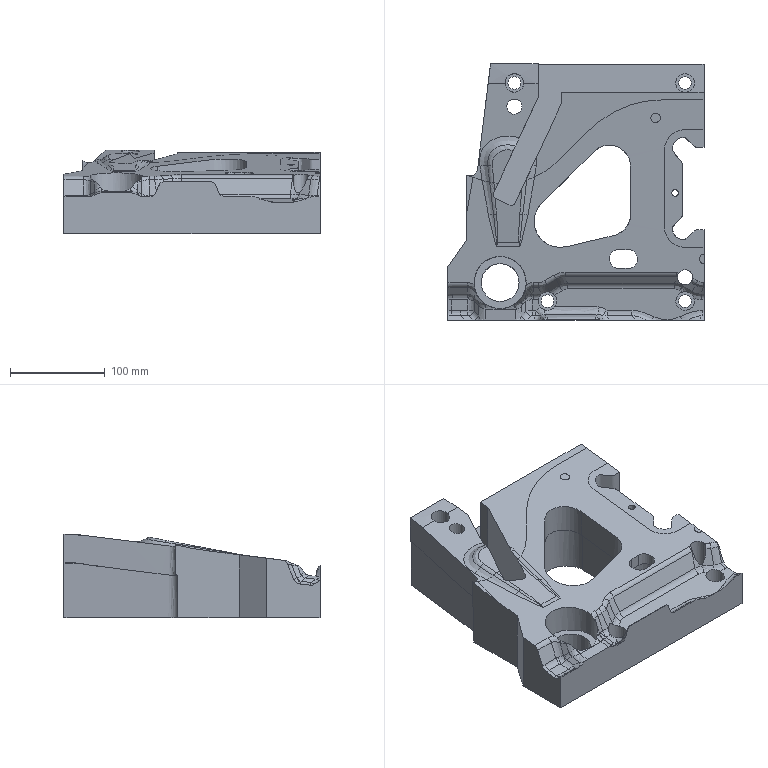Part | NX | features solid 2 | 1 solid | 195 faces | box 270 x 270.004 x 88.09 mm | volume 3116758 mm3 | spline 150 | plane 26 | cylinder 19 | commonest cylinder face diameters 13.5 x4 19.5 x4 10 x3 16 x2 20 x2 7 x1